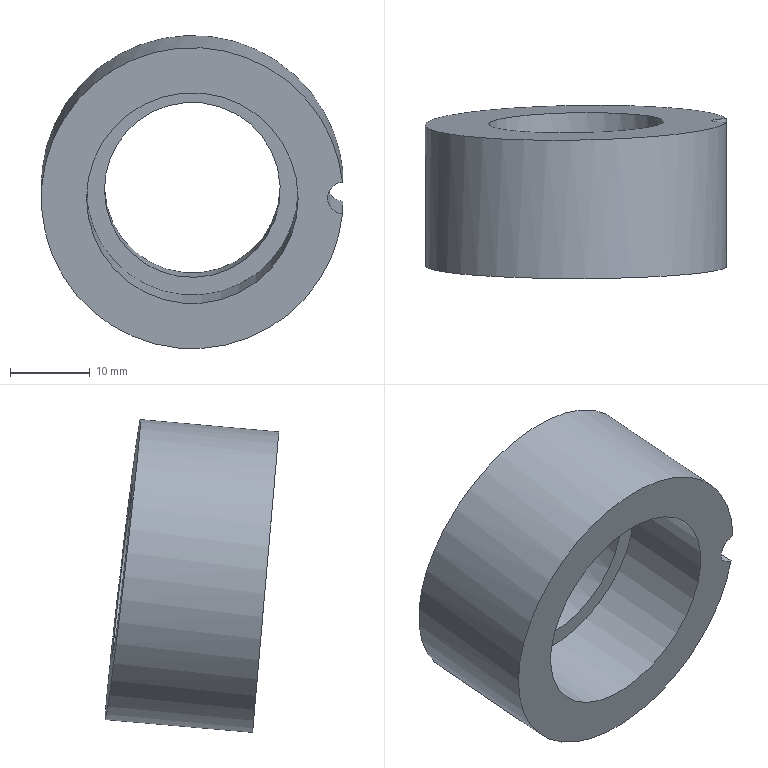Part | NX | features EKSD 38-20-22.10 2 | 1 solid | 7 faces | box 37.895 x 21.847 x 39.379 mm | volume 11356 mm3 | cylinder 4 | plane 3 | commonest cylinder face diameters 4 x1 22.1 x1 26.6 x1 38 x1
STEP:
#1=CARTESIAN_POINT('',(-131.293,40.21,-41.38));
#2=VERTEX_POINT('',#1);
#3=CARTESIAN_POINT('',(-131.293,39.862,-37.401));
#4=VERTEX_POINT('',#3);
#5=CARTESIAN_POINT('',(-131.187,40.036,-39.391));
#6=DIRECTION('',(0.,0.9962,0.08716));
#7=DIRECTION('',(-1.,0.,0.));
#8=AXIS2_PLACEMENT_3D('',#5,#6,#7);
#9=CIRCLE('',#8,2.);
#10=EDGE_CURVE('',#2,#4,#9,.T.);
#11=ORIENTED_EDGE('',*,*,#10,.T.);
#12=CARTESIAN_POINT('',(-150.187,40.036,-39.391));
#13=DIRECTION('',(0.,0.9962,0.08716));
#14=DIRECTION('',(-1.,0.,0.));
#15=AXIS2_PLACEMENT_3D('',#12,#13,#14);
#16=CIRCLE('',#15,19.);
#17=EDGE_CURVE('',#2,#4,#16,.T.);
#18=ORIENTED_EDGE('',*,*,#17,.F.);
#19=EDGE_LOOP('',(#11,#18));
#20=FACE_BOUND('',#19,.T.);
#21=CARTESIAN_POINT('',(-136.887,40.036,-39.391));
#22=VERTEX_POINT('',#21);
#23=CARTESIAN_POINT('',(-150.187,40.036,-39.391));
#24=DIRECTION('',(0.,-0.9962,-0.08716));
#25=DIRECTION('',(1.,0.,0.));
#26=AXIS2_PLACEMENT_3D('',#23,#24,#25);
#27=CIRCLE('',#26,13.3);
#28=EDGE_CURVE('',#22,#22,#27,.T.);
#29=ORIENTED_EDGE('',*,*,#28,.F.);
#30=EDGE_LOOP('',(#29));
#31=FACE_BOUND('',#30,.T.);
#32=CARTESIAN_POINT('',(-150.187,40.036,-39.391));
#33=DIRECTION('',(0.,-0.9962,-0.08716));
#34=DIRECTION('',(1.,0.,0.));
#35=AXIS2_PLACEMENT_3D('',#32,#33,#34);
#36=PLANE('',#35);
#37=ADVANCED_FACE('',(#20,#31),#36,.T.);
#38=CARTESIAN_POINT('',(-131.293,58.054,-35.809));
#39=VERTEX_POINT('',#38);
#40=CARTESIAN_POINT('',(-131.293,58.518,-39.778));
#41=VERTEX_POINT('',#40);
#42=CARTESIAN_POINT('',(-131.187,58.287,-37.794));
#43=DIRECTION('',(-0.01517,0.9931,0.1162));
#44=DIRECTION('',(-0.4611,-0.11,0.8805));
#45=AXIS2_PLACEMENT_3D('',#42,#43,#44);
#46=ELLIPSE('',#45,2.001,2.);
#47=EDGE_CURVE('',#39,#41,#46,.F.);
#48=ORIENTED_EDGE('',*,*,#47,.T.);
#49=CARTESIAN_POINT('',(-150.187,58.,-37.819));
#50=DIRECTION('',(-0.01517,0.9931,0.1162));
#51=DIRECTION('',(-0.4611,-0.11,0.8805));
#52=AXIS2_PLACEMENT_3D('',#49,#50,#51);
#53=ELLIPSE('',#52,19.01,19.);
#54=EDGE_CURVE('',#39,#41,#53,.F.);
#55=ORIENTED_EDGE('',*,*,#54,.F.);
#56=EDGE_LOOP('',(#48,#55));
#57=FACE_BOUND('',#56,.T.);
#58=CARTESIAN_POINT('',(-155.285,56.783,-28.084));
#59=VERTEX_POINT('',#58);
#60=CARTESIAN_POINT('',(-150.187,58.,-37.819));
#61=DIRECTION('',(-0.01517,0.9931,0.1162));
#62=DIRECTION('',(-0.4611,-0.11,0.8805));
#63=AXIS2_PLACEMENT_3D('',#60,#61,#62);
#64=ELLIPSE('',#63,11.056,11.05);
#65=EDGE_CURVE('',#59,#59,#64,.T.);
#66=ORIENTED_EDGE('',*,*,#65,.F.);
#67=EDGE_LOOP('',(#66));
#68=FACE_BOUND('',#67,.T.);
#69=CARTESIAN_POINT('',(-173.425,42.623,90.607));
#70=DIRECTION('',(-0.01517,0.9931,0.1162));
#71=DIRECTION('',(0.05188,0.1168,-0.9918));
#72=AXIS2_PLACEMENT_3D('',#69,#70,#71);
#73=PLANE('',#72);
#74=ADVANCED_FACE('',(#57,#68),#73,.T.);
#75=CARTESIAN_POINT('',(-131.293,49.824,-36.529));
#76=DIRECTION('',(0.,-0.9962,-0.08716));
#77=VECTOR('',#76,1000.);
#78=LINE('',#75,#77);
#79=EDGE_CURVE('',#39,#4,#78,.T.);
#80=ORIENTED_EDGE('',*,*,#79,.F.);
#81=ORIENTED_EDGE('',*,*,#54,.T.);
#82=CARTESIAN_POINT('',(-131.293,50.172,-40.509));
#83=DIRECTION('',(0.,-0.9962,-0.08716));
#84=VECTOR('',#83,1000.);
#85=LINE('',#82,#84);
#86=EDGE_CURVE('',#2,#41,#85,.F.);
#87=ORIENTED_EDGE('',*,*,#86,.F.);
#88=ORIENTED_EDGE('',*,*,#17,.T.);
#89=EDGE_LOOP('',(#80,#81,#87,#88));
#90=FACE_BOUND('',#89,.T.);
#91=CARTESIAN_POINT('',(-150.187,59.96,-37.647));
#92=DIRECTION('',(0.,-0.9962,-0.08716));
#93=DIRECTION('',(1.,0.,0.));
#94=AXIS2_PLACEMENT_3D('',#91,#92,#93);
#95=CYLINDRICAL_SURFACE('',#94,19.);
#96=ADVANCED_FACE('',(#90),#95,.T.);
#97=CARTESIAN_POINT('',(-161.237,51.991,-38.345));
#98=VERTEX_POINT('',#97);
#99=CARTESIAN_POINT('',(-150.187,51.991,-38.345));
#100=DIRECTION('',(0.,0.9962,0.08716));
#101=DIRECTION('',(-1.,0.,0.));
#102=AXIS2_PLACEMENT_3D('',#99,#100,#101);
#103=CIRCLE('',#102,11.05);
#104=EDGE_CURVE('',#98,#98,#103,.F.);
#105=ORIENTED_EDGE('',*,*,#104,.T.);
#106=EDGE_LOOP('',(#105));
#107=FACE_BOUND('',#106,.T.);
#108=ORIENTED_EDGE('',*,*,#65,.T.);
#109=EDGE_LOOP('',(#108));
#110=FACE_BOUND('',#109,.T.);
#111=CARTESIAN_POINT('',(-150.187,60.956,-37.56));
#112=DIRECTION('',(0.,-0.9962,-0.08716));
#113=DIRECTION('',(1.,0.,0.));
#114=AXIS2_PLACEMENT_3D('',#111,#112,#113);
#115=CYLINDRICAL_SURFACE('',#114,11.05);
#116=ADVANCED_FACE('',(#107,#110),#115,.F.);
#117=CARTESIAN_POINT('',(-136.887,51.991,-38.345));
#118=VERTEX_POINT('',#117);
#119=CARTESIAN_POINT('',(-150.187,51.991,-38.345));
#120=DIRECTION('',(0.,-0.9962,-0.08716));
#121=DIRECTION('',(1.,0.,0.));
#122=AXIS2_PLACEMENT_3D('',#119,#120,#121);
#123=CIRCLE('',#122,13.3);
#124=EDGE_CURVE('',#118,#118,#123,.T.);
#125=ORIENTED_EDGE('',*,*,#124,.T.);
#126=EDGE_LOOP('',(#125));
#127=FACE_BOUND('',#126,.T.);
#128=ORIENTED_EDGE('',*,*,#104,.F.);
#129=EDGE_LOOP('',(#128));
#130=FACE_BOUND('',#129,.T.);
#131=CARTESIAN_POINT('',(-150.187,51.991,-38.345));
#132=DIRECTION('',(0.,0.9962,0.08716));
#133=DIRECTION('',(-1.,0.,0.));
#134=AXIS2_PLACEMENT_3D('',#131,#132,#133);
#135=PLANE('',#134);
#136=ADVANCED_FACE('',(#127,#130),#135,.F.);
#137=ORIENTED_EDGE('',*,*,#28,.T.);
#138=EDGE_LOOP('',(#137));
#139=FACE_BOUND('',#138,.T.);
#140=ORIENTED_EDGE('',*,*,#124,.F.);
#141=EDGE_LOOP('',(#140));
#142=FACE_BOUND('',#141,.T.);
#143=CARTESIAN_POINT('',(-150.187,51.991,-38.345));
#144=DIRECTION('',(0.,-0.9962,-0.08716));
#145=DIRECTION('',(1.,0.,0.));
#146=AXIS2_PLACEMENT_3D('',#143,#144,#145);
#147=CYLINDRICAL_SURFACE('',#146,13.3);
#148=ADVANCED_FACE('',(#139,#142),#147,.F.);
#149=ORIENTED_EDGE('',*,*,#79,.T.);
#150=ORIENTED_EDGE('',*,*,#10,.F.);
#151=ORIENTED_EDGE('',*,*,#86,.T.);
#152=ORIENTED_EDGE('',*,*,#47,.F.);
#153=EDGE_LOOP('',(#149,#150,#151,#152));
#154=FACE_BOUND('',#153,.T.);
#155=CARTESIAN_POINT('',(-131.187,59.96,-37.647));
#156=DIRECTION('',(0.,-0.9962,-0.08716));
#157=DIRECTION('',(1.,0.,0.));
#158=AXIS2_PLACEMENT_3D('',#155,#156,#157);
#159=CYLINDRICAL_SURFACE('',#158,2.);
#160=ADVANCED_FACE('',(#154),#159,.F.);
#161=CLOSED_SHELL('',(#37,#74,#96,#116,#136,#148,#160));
#162=MANIFOLD_SOLID_BREP('',#161);
#163=(LENGTH_UNIT()NAMED_UNIT(*)SI_UNIT(.MILLI.,.METRE.));
#164=UNCERTAINTY_MEASURE_WITH_UNIT(LENGTH_MEASURE(0.00001),#163,'','');
#165=(NAMED_UNIT(*)PLANE_ANGLE_UNIT()SI_UNIT($,.RADIAN.));
#166=(NAMED_UNIT(*)SI_UNIT($,.STERADIAN.)SOLID_ANGLE_UNIT());
#167=(GEOMETRIC_REPRESENTATION_CONTEXT(3)GLOBAL_UNCERTAINTY_ASSIGNED_CONTEXT((#164))GLOBAL_UNIT_ASSIGNED_CONTEXT((#163,#165,#166))REPRESENTATION_CONTEXT('',''));
#168=ADVANCED_BREP_SHAPE_REPRESENTATION('',(#162),#167);